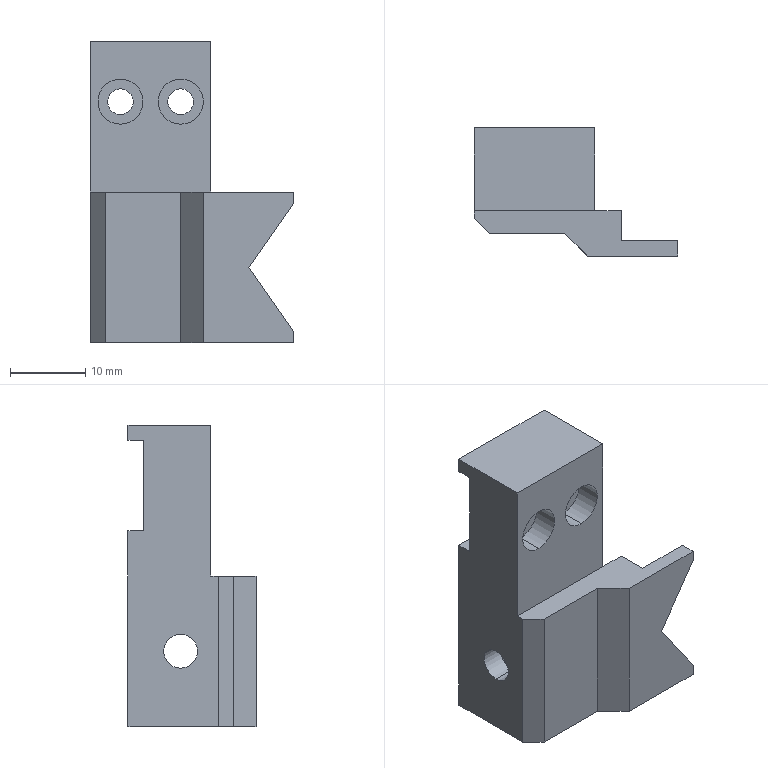Part | STEP file | PN_0015 | 1 solid | 46 faces | box 27 x 17 x 40 mm | volume 6793 mm3 | plane 28 | cylinder 14 | cone 4 | commonest cylinder face diameters 3.4 x4 4.4 x4 6 x4 4.5 x2